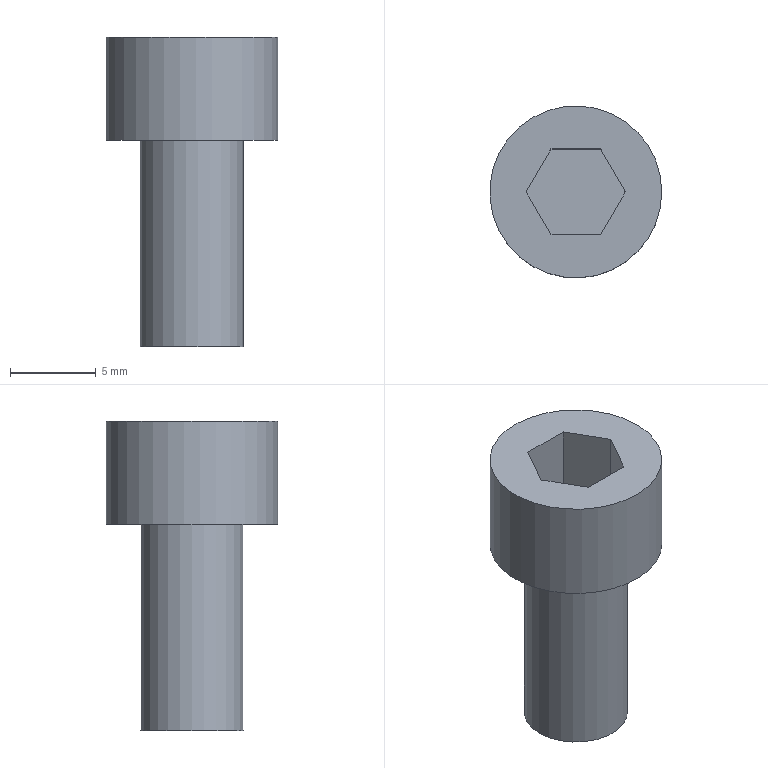Part | STEP file | lll_id750_x_t | 1 solid | 12 faces | box 10 x 10 x 18 mm | volume 724.794 mm3 | plane 10 | cylinder 2 | commonest cylinder face diameters 6 x1 10 x1
STEP:
#1=CARTESIAN_POINT('',(75.,65.,-12.5));
#2=VERTEX_POINT('',#1);
#3=CARTESIAN_POINT('',(70.,65.,-12.5));
#4=DIRECTION('',(0.,0.,1.));
#5=DIRECTION('',(1.,0.,0.));
#6=AXIS2_PLACEMENT_3D('',#3,#4,#5);
#7=CIRCLE('',#6,5.);
#8=EDGE_CURVE('',#2,#2,#7,.T.);
#9=ORIENTED_EDGE('',*,*,#8,.T.);
#10=EDGE_LOOP('',(#9));
#11=FACE_BOUND('',#10,.T.);
#12=CARTESIAN_POINT('',(68.557,67.5,-12.5));
#13=VERTEX_POINT('',#12);
#14=CARTESIAN_POINT('',(71.443,67.5,-12.5));
#15=VERTEX_POINT('',#14);
#16=CARTESIAN_POINT('',(68.557,67.5,-12.5));
#17=DIRECTION('',(1.,0.,0.));
#18=VECTOR('',#17,1.);
#19=LINE('',#16,#18);
#20=EDGE_CURVE('',#13,#15,#19,.T.);
#21=ORIENTED_EDGE('',*,*,#20,.T.);
#22=CARTESIAN_POINT('',(72.887,65.,-12.5));
#23=VERTEX_POINT('',#22);
#24=CARTESIAN_POINT('',(71.443,67.5,-12.5));
#25=DIRECTION('',(0.5,-0.866,0.));
#26=VECTOR('',#25,1.);
#27=LINE('',#24,#26);
#28=EDGE_CURVE('',#15,#23,#27,.T.);
#29=ORIENTED_EDGE('',*,*,#28,.T.);
#30=CARTESIAN_POINT('',(71.443,62.5,-12.5));
#31=VERTEX_POINT('',#30);
#32=CARTESIAN_POINT('',(72.887,65.,-12.5));
#33=DIRECTION('',(-0.5,-0.866,0.));
#34=VECTOR('',#33,1.);
#35=LINE('',#32,#34);
#36=EDGE_CURVE('',#23,#31,#35,.T.);
#37=ORIENTED_EDGE('',*,*,#36,.T.);
#38=CARTESIAN_POINT('',(68.557,62.5,-12.5));
#39=VERTEX_POINT('',#38);
#40=CARTESIAN_POINT('',(71.443,62.5,-12.5));
#41=DIRECTION('',(-1.,0.,0.));
#42=VECTOR('',#41,1.);
#43=LINE('',#40,#42);
#44=EDGE_CURVE('',#31,#39,#43,.T.);
#45=ORIENTED_EDGE('',*,*,#44,.T.);
#46=CARTESIAN_POINT('',(67.113,65.,-12.5));
#47=VERTEX_POINT('',#46);
#48=CARTESIAN_POINT('',(68.557,62.5,-12.5));
#49=DIRECTION('',(-0.5,0.866,0.));
#50=VECTOR('',#49,1.);
#51=LINE('',#48,#50);
#52=EDGE_CURVE('',#39,#47,#51,.T.);
#53=ORIENTED_EDGE('',*,*,#52,.T.);
#54=CARTESIAN_POINT('',(67.113,65.,-12.5));
#55=DIRECTION('',(0.5,0.866,0.));
#56=VECTOR('',#55,1.);
#57=LINE('',#54,#56);
#58=EDGE_CURVE('',#47,#13,#57,.T.);
#59=ORIENTED_EDGE('',*,*,#58,.T.);
#60=EDGE_LOOP('',(#21,#29,#37,#45,#53,#59));
#61=FACE_BOUND('',#60,.T.);
#62=CARTESIAN_POINT('',(75.,65.,-12.5));
#63=DIRECTION('',(0.,0.,-1.));
#64=DIRECTION('',(-1.,0.,0.));
#65=AXIS2_PLACEMENT_3D('',#62,#63,#64);
#66=PLANE('',#65);
#67=ADVANCED_FACE('',(#11,#61),#66,.F.);
#68=ORIENTED_EDGE('',*,*,#8,.F.);
#69=EDGE_LOOP('',(#68));
#70=FACE_BOUND('',#69,.T.);
#71=CARTESIAN_POINT('',(75.,65.,-18.5));
#72=VERTEX_POINT('',#71);
#73=CARTESIAN_POINT('',(70.,65.,-18.5));
#74=DIRECTION('',(0.,0.,1.));
#75=DIRECTION('',(1.,0.,0.));
#76=AXIS2_PLACEMENT_3D('',#73,#74,#75);
#77=CIRCLE('',#76,5.);
#78=EDGE_CURVE('',#72,#72,#77,.T.);
#79=ORIENTED_EDGE('',*,*,#78,.T.);
#80=EDGE_LOOP('',(#79));
#81=FACE_BOUND('',#80,.T.);
#82=CARTESIAN_POINT('',(70.,65.,-18.4));
#83=DIRECTION('',(0.,0.,1.));
#84=DIRECTION('',(1.,0.,0.));
#85=AXIS2_PLACEMENT_3D('',#82,#83,#84);
#86=CYLINDRICAL_SURFACE('',#85,5.);
#87=ADVANCED_FACE('',(#70,#81),#86,.T.);
#88=ORIENTED_EDGE('',*,*,#78,.F.);
#89=EDGE_LOOP('',(#88));
#90=FACE_BOUND('',#89,.T.);
#91=CARTESIAN_POINT('',(73.,65.,-18.5));
#92=VERTEX_POINT('',#91);
#93=CARTESIAN_POINT('',(70.,65.,-18.5));
#94=DIRECTION('',(0.,0.,1.));
#95=DIRECTION('',(1.,0.,0.));
#96=AXIS2_PLACEMENT_3D('',#93,#94,#95);
#97=CIRCLE('',#96,3.);
#98=EDGE_CURVE('',#92,#92,#97,.T.);
#99=ORIENTED_EDGE('',*,*,#98,.T.);
#100=EDGE_LOOP('',(#99));
#101=FACE_BOUND('',#100,.T.);
#102=CARTESIAN_POINT('',(73.,65.,-18.5));
#103=DIRECTION('',(0.,0.,1.));
#104=DIRECTION('',(1.,0.,0.));
#105=AXIS2_PLACEMENT_3D('',#102,#103,#104);
#106=PLANE('',#105);
#107=ADVANCED_FACE('',(#90,#101),#106,.F.);
#108=ORIENTED_EDGE('',*,*,#98,.F.);
#109=EDGE_LOOP('',(#108));
#110=FACE_BOUND('',#109,.T.);
#111=CARTESIAN_POINT('',(73.,65.,-30.5));
#112=VERTEX_POINT('',#111);
#113=CARTESIAN_POINT('',(70.,65.,-30.5));
#114=DIRECTION('',(0.,0.,1.));
#115=DIRECTION('',(1.,0.,0.));
#116=AXIS2_PLACEMENT_3D('',#113,#114,#115);
#117=CIRCLE('',#116,3.);
#118=EDGE_CURVE('',#112,#112,#117,.T.);
#119=ORIENTED_EDGE('',*,*,#118,.T.);
#120=EDGE_LOOP('',(#119));
#121=FACE_BOUND('',#120,.T.);
#122=CARTESIAN_POINT('',(70.,65.,-18.4));
#123=DIRECTION('',(0.,0.,1.));
#124=DIRECTION('',(1.,0.,0.));
#125=AXIS2_PLACEMENT_3D('',#122,#123,#124);
#126=CYLINDRICAL_SURFACE('',#125,3.);
#127=ADVANCED_FACE('',(#110,#121),#126,.T.);
#128=ORIENTED_EDGE('',*,*,#118,.F.);
#129=EDGE_LOOP('',(#128));
#130=FACE_OUTER_BOUND('',#129,.T.);
#131=CARTESIAN_POINT('',(70.,65.,-30.5));
#132=DIRECTION('',(0.,0.,1.));
#133=DIRECTION('',(1.,0.,0.));
#134=AXIS2_PLACEMENT_3D('',#131,#132,#133);
#135=PLANE('',#134);
#136=ADVANCED_FACE('',(#130),#135,.F.);
#137=ORIENTED_EDGE('',*,*,#20,.F.);
#138=CARTESIAN_POINT('',(68.557,67.5,-16.46));
#139=VERTEX_POINT('',#138);
#140=CARTESIAN_POINT('',(68.557,67.5,-16.46));
#141=DIRECTION('',(0.,0.,-1.));
#142=VECTOR('',#141,1.);
#143=LINE('',#140,#142);
#144=EDGE_CURVE('',#13,#139,#143,.T.);
#145=ORIENTED_EDGE('',*,*,#144,.T.);
#146=CARTESIAN_POINT('',(71.443,67.5,-16.46));
#147=VERTEX_POINT('',#146);
#148=CARTESIAN_POINT('',(68.557,67.5,-16.46));
#149=DIRECTION('',(-1.,0.,0.));
#150=VECTOR('',#149,1.);
#151=LINE('',#148,#150);
#152=EDGE_CURVE('',#147,#139,#151,.T.);
#153=ORIENTED_EDGE('',*,*,#152,.F.);
#154=CARTESIAN_POINT('',(71.443,67.5,-16.46));
#155=DIRECTION('',(0.,0.,-1.));
#156=VECTOR('',#155,1.);
#157=LINE('',#154,#156);
#158=EDGE_CURVE('',#15,#147,#157,.T.);
#159=ORIENTED_EDGE('',*,*,#158,.F.);
#160=EDGE_LOOP('',(#137,#145,#153,#159));
#161=FACE_OUTER_BOUND('',#160,.T.);
#162=CARTESIAN_POINT('',(68.557,67.5,-16.46));
#163=DIRECTION('',(0.,-1.,0.));
#164=DIRECTION('',(1.,0.,0.));
#165=AXIS2_PLACEMENT_3D('',#162,#163,#164);
#166=PLANE('',#165);
#167=ADVANCED_FACE('',(#161),#166,.T.);
#168=ORIENTED_EDGE('',*,*,#28,.F.);
#169=ORIENTED_EDGE('',*,*,#158,.T.);
#170=CARTESIAN_POINT('',(72.887,65.,-16.46));
#171=VERTEX_POINT('',#170);
#172=CARTESIAN_POINT('',(71.443,67.5,-16.46));
#173=DIRECTION('',(-0.5,0.866,0.));
#174=VECTOR('',#173,1.);
#175=LINE('',#172,#174);
#176=EDGE_CURVE('',#171,#147,#175,.T.);
#177=ORIENTED_EDGE('',*,*,#176,.F.);
#178=CARTESIAN_POINT('',(72.887,65.,-16.46));
#179=DIRECTION('',(0.,0.,-1.));
#180=VECTOR('',#179,1.);
#181=LINE('',#178,#180);
#182=EDGE_CURVE('',#23,#171,#181,.T.);
#183=ORIENTED_EDGE('',*,*,#182,.F.);
#184=EDGE_LOOP('',(#168,#169,#177,#183));
#185=FACE_OUTER_BOUND('',#184,.T.);
#186=CARTESIAN_POINT('',(71.443,67.5,-16.46));
#187=DIRECTION('',(-0.866,-0.5,0.));
#188=DIRECTION('',(0.5,-0.866,0.));
#189=AXIS2_PLACEMENT_3D('',#186,#187,#188);
#190=PLANE('',#189);
#191=ADVANCED_FACE('',(#185),#190,.T.);
#192=ORIENTED_EDGE('',*,*,#36,.F.);
#193=ORIENTED_EDGE('',*,*,#182,.T.);
#194=CARTESIAN_POINT('',(71.443,62.5,-16.46));
#195=VERTEX_POINT('',#194);
#196=CARTESIAN_POINT('',(72.887,65.,-16.46));
#197=DIRECTION('',(0.5,0.866,0.));
#198=VECTOR('',#197,1.);
#199=LINE('',#196,#198);
#200=EDGE_CURVE('',#195,#171,#199,.T.);
#201=ORIENTED_EDGE('',*,*,#200,.F.);
#202=CARTESIAN_POINT('',(71.443,62.5,-16.46));
#203=DIRECTION('',(0.,0.,-1.));
#204=VECTOR('',#203,1.);
#205=LINE('',#202,#204);
#206=EDGE_CURVE('',#31,#195,#205,.T.);
#207=ORIENTED_EDGE('',*,*,#206,.F.);
#208=EDGE_LOOP('',(#192,#193,#201,#207));
#209=FACE_OUTER_BOUND('',#208,.T.);
#210=CARTESIAN_POINT('',(72.887,65.,-16.46));
#211=DIRECTION('',(-0.866,0.5,0.));
#212=DIRECTION('',(-0.5,-0.866,0.));
#213=AXIS2_PLACEMENT_3D('',#210,#211,#212);
#214=PLANE('',#213);
#215=ADVANCED_FACE('',(#209),#214,.T.);
#216=ORIENTED_EDGE('',*,*,#44,.F.);
#217=ORIENTED_EDGE('',*,*,#206,.T.);
#218=CARTESIAN_POINT('',(68.557,62.5,-16.46));
#219=VERTEX_POINT('',#218);
#220=CARTESIAN_POINT('',(71.443,62.5,-16.46));
#221=DIRECTION('',(1.,0.,0.));
#222=VECTOR('',#221,1.);
#223=LINE('',#220,#222);
#224=EDGE_CURVE('',#219,#195,#223,.T.);
#225=ORIENTED_EDGE('',*,*,#224,.F.);
#226=CARTESIAN_POINT('',(68.557,62.5,-16.46));
#227=DIRECTION('',(0.,0.,-1.));
#228=VECTOR('',#227,1.);
#229=LINE('',#226,#228);
#230=EDGE_CURVE('',#39,#219,#229,.T.);
#231=ORIENTED_EDGE('',*,*,#230,.F.);
#232=EDGE_LOOP('',(#216,#217,#225,#231));
#233=FACE_OUTER_BOUND('',#232,.T.);
#234=CARTESIAN_POINT('',(71.443,62.5,-16.46));
#235=DIRECTION('',(0.,1.,0.));
#236=DIRECTION('',(-1.,0.,0.));
#237=AXIS2_PLACEMENT_3D('',#234,#235,#236);
#238=PLANE('',#237);
#239=ADVANCED_FACE('',(#233),#238,.T.);
#240=ORIENTED_EDGE('',*,*,#52,.F.);
#241=ORIENTED_EDGE('',*,*,#230,.T.);
#242=CARTESIAN_POINT('',(67.113,65.,-16.46));
#243=VERTEX_POINT('',#242);
#244=CARTESIAN_POINT('',(68.557,62.5,-16.46));
#245=DIRECTION('',(0.5,-0.866,0.));
#246=VECTOR('',#245,1.);
#247=LINE('',#244,#246);
#248=EDGE_CURVE('',#243,#219,#247,.T.);
#249=ORIENTED_EDGE('',*,*,#248,.F.);
#250=CARTESIAN_POINT('',(67.113,65.,-16.46));
#251=DIRECTION('',(0.,0.,-1.));
#252=VECTOR('',#251,1.);
#253=LINE('',#250,#252);
#254=EDGE_CURVE('',#47,#243,#253,.T.);
#255=ORIENTED_EDGE('',*,*,#254,.F.);
#256=EDGE_LOOP('',(#240,#241,#249,#255));
#257=FACE_OUTER_BOUND('',#256,.T.);
#258=CARTESIAN_POINT('',(68.557,62.5,-16.46));
#259=DIRECTION('',(0.866,0.5,0.));
#260=DIRECTION('',(-0.5,0.866,0.));
#261=AXIS2_PLACEMENT_3D('',#258,#259,#260);
#262=PLANE('',#261);
#263=ADVANCED_FACE('',(#257),#262,.T.);
#264=ORIENTED_EDGE('',*,*,#58,.F.);
#265=ORIENTED_EDGE('',*,*,#254,.T.);
#266=CARTESIAN_POINT('',(67.113,65.,-16.46));
#267=DIRECTION('',(-0.5,-0.866,0.));
#268=VECTOR('',#267,1.);
#269=LINE('',#266,#268);
#270=EDGE_CURVE('',#139,#243,#269,.T.);
#271=ORIENTED_EDGE('',*,*,#270,.F.);
#272=ORIENTED_EDGE('',*,*,#144,.F.);
#273=EDGE_LOOP('',(#264,#265,#271,#272));
#274=FACE_OUTER_BOUND('',#273,.T.);
#275=CARTESIAN_POINT('',(67.113,65.,-16.46));
#276=DIRECTION('',(0.866,-0.5,0.));
#277=DIRECTION('',(0.5,0.866,0.));
#278=AXIS2_PLACEMENT_3D('',#275,#276,#277);
#279=PLANE('',#278);
#280=ADVANCED_FACE('',(#274),#279,.T.);
#281=ORIENTED_EDGE('',*,*,#152,.T.);
#282=ORIENTED_EDGE('',*,*,#270,.T.);
#283=ORIENTED_EDGE('',*,*,#248,.T.);
#284=ORIENTED_EDGE('',*,*,#224,.T.);
#285=ORIENTED_EDGE('',*,*,#200,.T.);
#286=ORIENTED_EDGE('',*,*,#176,.T.);
#287=EDGE_LOOP('',(#281,#282,#283,#284,#285,#286));
#288=FACE_OUTER_BOUND('',#287,.T.);
#289=CARTESIAN_POINT('',(70.,65.,-16.46));
#290=DIRECTION('',(0.,0.,-1.));
#291=DIRECTION('',(-1.,0.,0.));
#292=AXIS2_PLACEMENT_3D('',#289,#290,#291);
#293=PLANE('',#292);
#294=ADVANCED_FACE('',(#288),#293,.F.);
#295=CLOSED_SHELL('',(#67,#87,#107,#127,#136,#167,#191,#215,#239,#263,#280,#294));
#296=MANIFOLD_SOLID_BREP('',#295);
#297=(LENGTH_UNIT()NAMED_UNIT(*)SI_UNIT(.MILLI.,.METRE.));
#298=UNCERTAINTY_MEASURE_WITH_UNIT(LENGTH_MEASURE(0.00002),#297,'','');
#299=(NAMED_UNIT(*)PLANE_ANGLE_UNIT()SI_UNIT($,.RADIAN.));
#300=PLANE_ANGLE_MEASURE_WITH_UNIT(PLANE_ANGLE_MEASURE(0.01745),#299);
#301=DIMENSIONAL_EXPONENTS(0.,0.,0.,0.,0.,0.,0.);
#302=(CONVERSION_BASED_UNIT('DEGREE',#300)NAMED_UNIT(#301)PLANE_ANGLE_UNIT());
#303=(NAMED_UNIT(*)SI_UNIT($,.STERADIAN.)SOLID_ANGLE_UNIT());
#304=(GEOMETRIC_REPRESENTATION_CONTEXT(3)GLOBAL_UNCERTAINTY_ASSIGNED_CONTEXT((#298))GLOBAL_UNIT_ASSIGNED_CONTEXT((#297,#302,#303))REPRESENTATION_CONTEXT('',''));
#305=ADVANCED_BREP_SHAPE_REPRESENTATION('',(#296),#304);